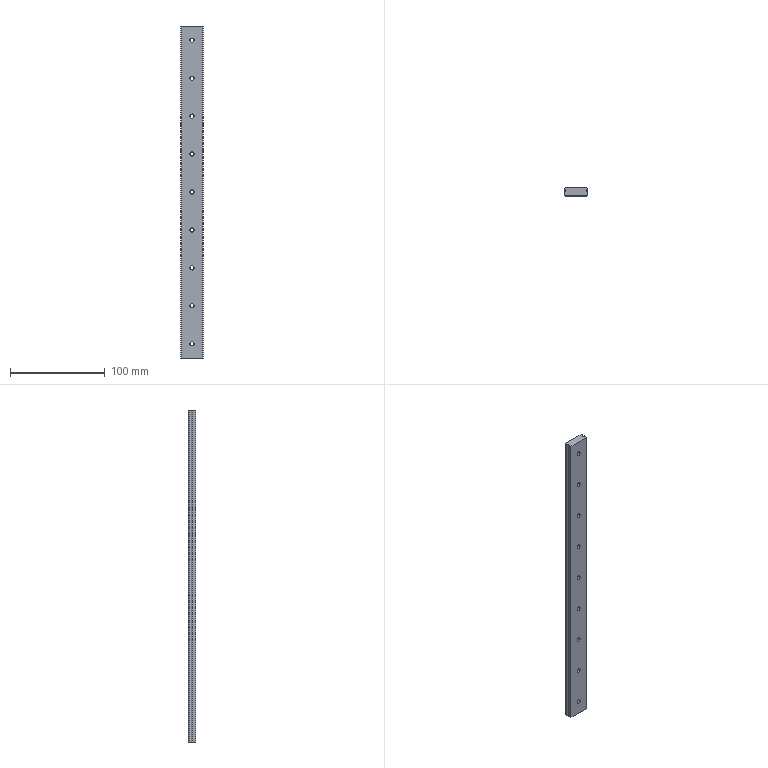Part | STEP file | 350 | 1 solid | 60 faces | box 24 x 8 x 350 mm | volume 62774 mm3 | cylinder 39 | plane 21 | commonest cylinder face diameters 4.5 x18 8 x18 2.5 x3